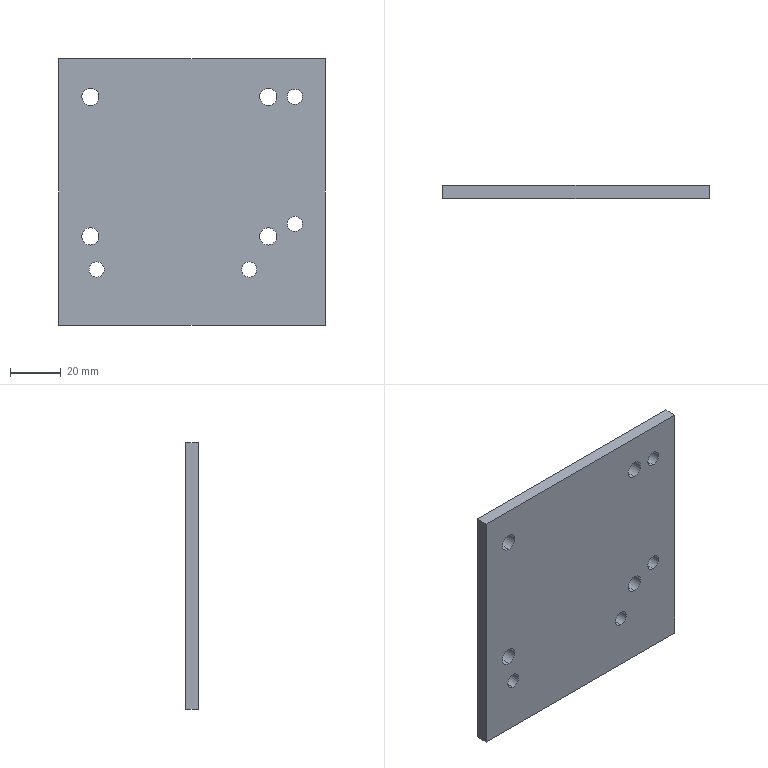Part | STEP file | 1 solid | 22 faces | box 105 x 5 x 105 mm | volume 53833 mm3 | cylinder 16 | plane 6 | commonest cylinder face diameters 6 x8 6.8 x8